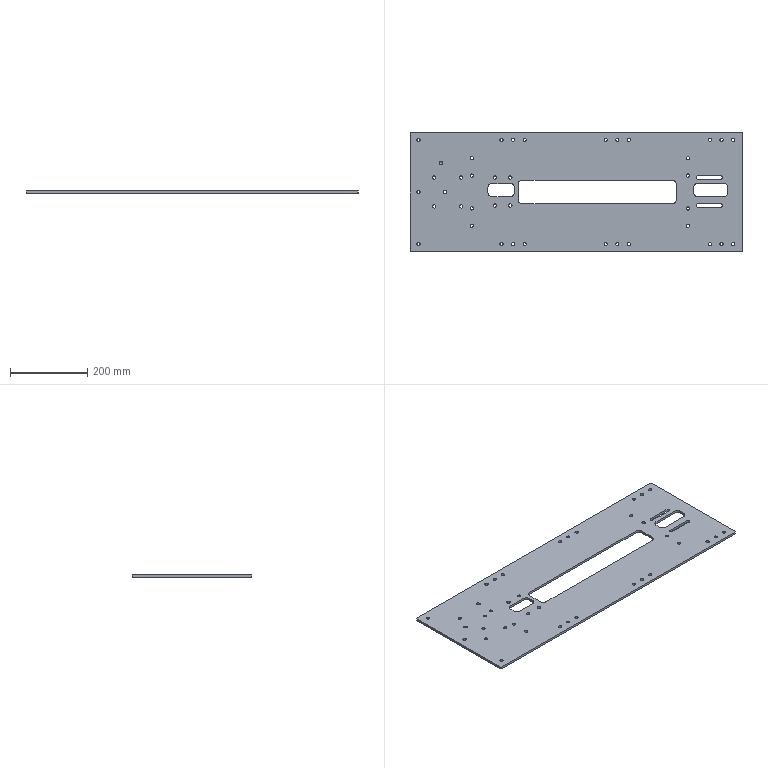Part | STEP file | 20301 | 1 solid | 122 faces | box 860 x 310 x 6 mm | volume 1402017 mm3 | cylinder 94 | plane 26 | cone 2 | commonest cylinder face diameters 8.5 x78 20 x12 8.2 x4